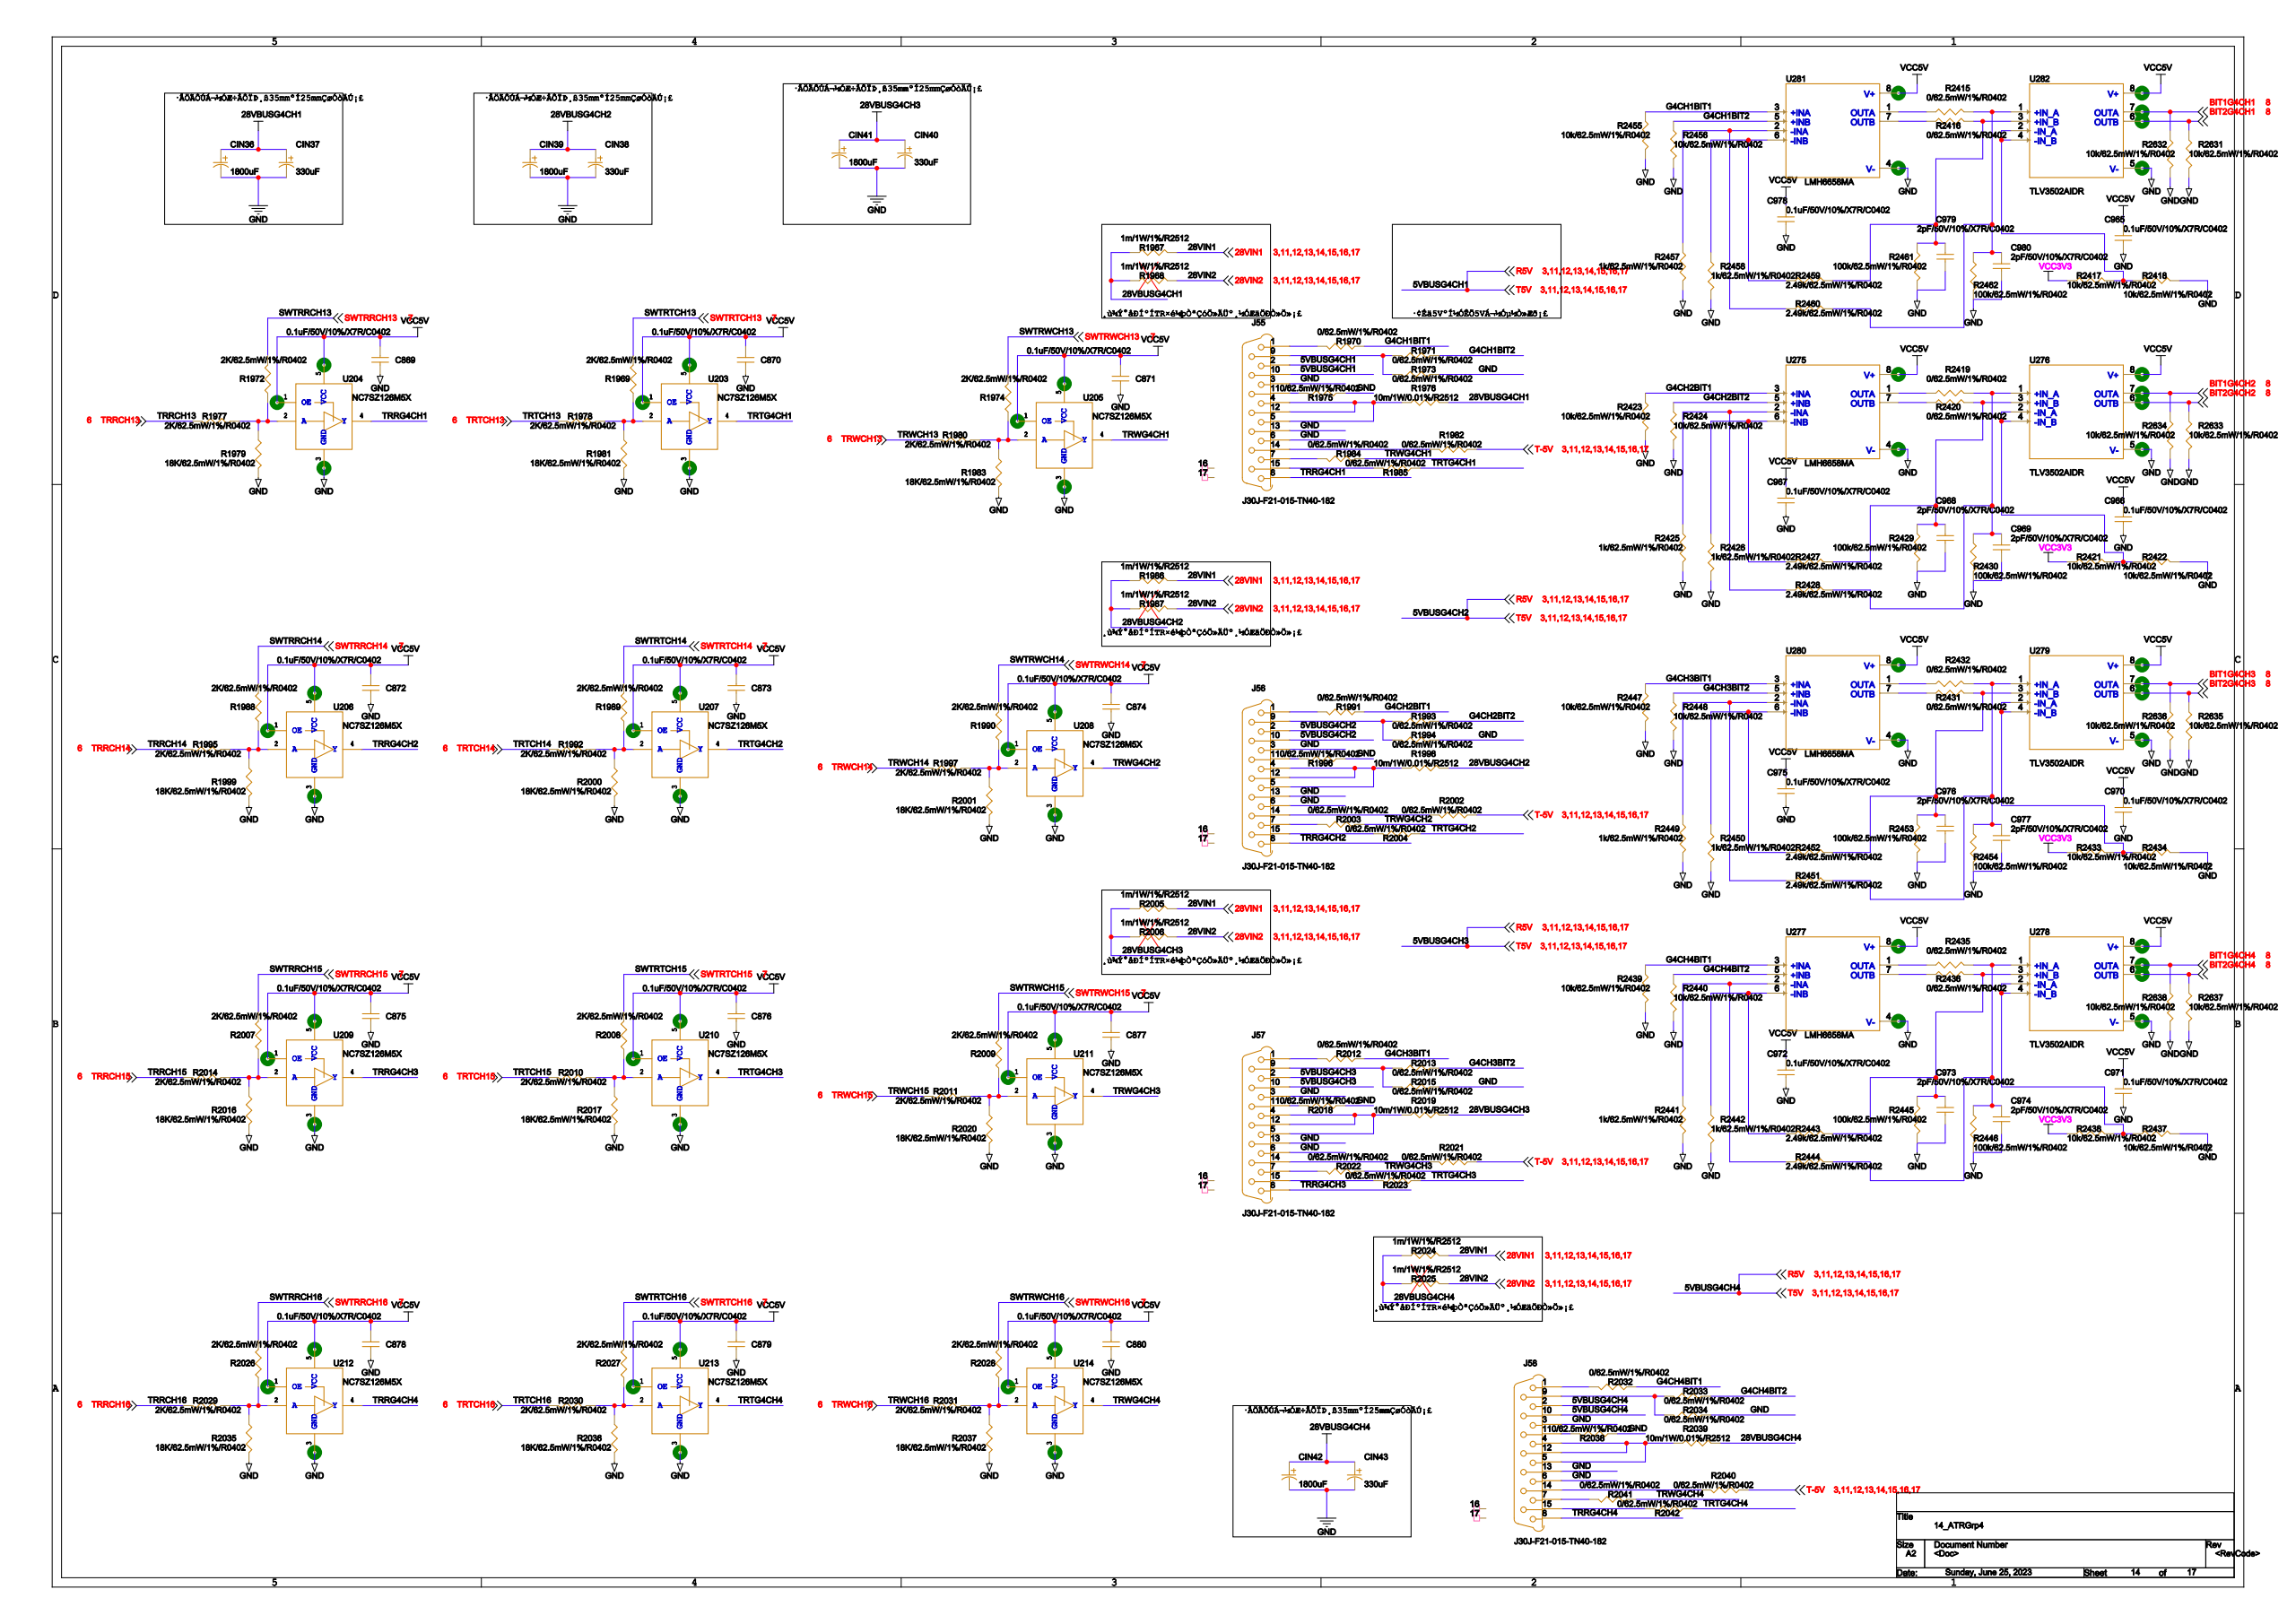Circuit board | Cadence Allegro | 1997 parts | 1536 nets | one sheet of the schematic
Parts on this sheet (reference | value | footprint):
C869 | 0.1uF/50V/10%/X7R/C0402 | 0402
C870 | 0.1uF/50V/10%/X7R/C0402 | 0402
C871 | 0.1uF/50V/10%/X7R/C0402 | 0402
C872 | 0.1uF/50V/10%/X7R/C0402 | 0402
C873 | 0.1uF/50V/10%/X7R/C0402 | 0402
C874 | 0.1uF/50V/10%/X7R/C0402 | 0402
C875 | 0.1uF/50V/10%/X7R/C0402 | 0402
C876 | 0.1uF/50V/10%/X7R/C0402 | 0402
C877 | 0.1uF/50V/10%/X7R/C0402 | 0402
C878 | 0.1uF/50V/10%/X7R/C0402 | 0402
C879 | 0.1uF/50V/10%/X7R/C0402 | 0402
C880 | 0.1uF/50V/10%/X7R/C0402 | 0402
C965 | 0.1uF/50V/10%/X7R/C0402 | 0402
C966 | 0.1uF/50V/10%/X7R/C0402 | 0402
C968 | 2pF/50V/10%/X7R/C0402 | 0402
C969 | 2pF/50V/10%/X7R/C0402 | 0402
C970 | 0.1uF/50V/10%/X7R/C0402 | 0402
C971 | 0.1uF/50V/10%/X7R/C0402 | 0402
C973 | 2pF/50V/10%/X7R/C0402 | 0402
C974 | 2pF/50V/10%/X7R/C0402 | 0402
C976 | 2pF/50V/10%/X7R/C0402 | 0402
C977 | 2pF/50V/10%/X7R/C0402 | 0402
C979 | 2pF/50V/10%/X7R/C0402 | 0402
C980 | 2pF/50V/10%/X7R/C0402 | 0402
CIN36 | ECF1HM182M27OTPO | AP-SMD_BD18-L27-W6_6-LS7_21
CIN37 | ECF1JM331G20OTPO | AP-SMD_BD10-L20-W6_6-LS7_21
CIN38 | ECF1JM331G20OTPO | AP-SMD_BD10-L20-W6_6-LS7_21
CIN39 | ECF1HM182M27OTPO | AP-SMD_BD18-L27-W6_6-LS7_21
CIN40 | ECF1JM331G20OTPO | AP-SMD_BD10-L20-W6_6-LS7_21
CIN41 | ECF1HM182M27OTPO | AP-SMD_BD18-L27-W6_6-LS7_21
CIN42 | ECF1HM182M27OTPO | AP-SMD_BD18-L27-W6_6-LS7_21
CIN43 | ECF1JM331G20OTPO | AP-SMD_BD10-L20-W6_6-LS7_21
J55 | J30J-F21-015-TN40-182 | J30J-F21-015-TN40-182
J56 | J30J-F21-015-TN40-182 | J30J-F21-015-TN40-182
J57 | J30J-F21-015-TN40-182 | J30J-F21-015-TN40-182
J58 | J30J-F21-015-TN40-182 | J30J-F21-015-TN40-182
R1967 | 1m/1W/1%/R2512 | 2512
R1968 | 1m/1W/1%/R2512 | 2512
R1969 | 2K/62.5mW/1%/R0402 | 0402
R1970 | 0/62.5mW/1%/R0402 | 0402
R1971 | 0/62.5mW/1%/R0402 | 0402
R1972 | 2K/62.5mW/1%/R0402 | 0402
R1973 | 0/62.5mW/1%/R0402 | 0402
R1974 | 2K/62.5mW/1%/R0402 | 0402
R1975 | 0/62.5mW/1%/R0402 | 0402
R1976 | 10m/1W/0.01%/R2512 | 2512
R1977 | 2K/62.5mW/1%/R0402 | 0402
R1978 | 2K/62.5mW/1%/R0402 | 0402
R1979 | 18K/62.5mW/1%/R0402 | 0402
R1980 | 2K/62.5mW/1%/R0402 | 0402
R1981 | 18K/62.5mW/1%/R0402 | 0402
R1982 | 0/62.5mW/1%/R0402 | 0402
R1983 | 18K/62.5mW/1%/R0402 | 0402
R1984 | 0/62.5mW/1%/R0402 | 0402
R1985 | 0/62.5mW/1%/R0402 | 0402
R1986 | 1m/1W/1%/R2512 | 2512
R1987 | 1m/1W/1%/R2512 | 2512
R1988 | 2K/62.5mW/1%/R0402 | 0402
R1989 | 2K/62.5mW/1%/R0402 | 0402
R1990 | 2K/62.5mW/1%/R0402 | 0402
R1991 | 0/62.5mW/1%/R0402 | 0402
R1992 | 2K/62.5mW/1%/R0402 | 0402
R1993 | 0/62.5mW/1%/R0402 | 0402
R1994 | 0/62.5mW/1%/R0402 | 0402
R1995 | 2K/62.5mW/1%/R0402 | 0402
R1996 | 0/62.5mW/1%/R0402 | 0402
R1997 | 2K/62.5mW/1%/R0402 | 0402
R1998 | 10m/1W/0.01%/R2512 | 2512
R1999 | 18K/62.5mW/1%/R0402 | 0402
R2000 | 18K/62.5mW/1%/R0402 | 0402
R2001 | 18K/62.5mW/1%/R0402 | 0402
R2002 | 0/62.5mW/1%/R0402 | 0402
R2003 | 0/62.5mW/1%/R0402 | 0402
R2004 | 0/62.5mW/1%/R0402 | 0402
R2005 | 1m/1W/1%/R2512 | 2512
R2006 | 1m/1W/1%/R2512 | 2512
R2007 | 2K/62.5mW/1%/R0402 | 0402
R2008 | 2K/62.5mW/1%/R0402 | 0402
R2009 | 2K/62.5mW/1%/R0402 | 0402
R2010 | 2K/62.5mW/1%/R0402 | 0402
R2011 | 2K/62.5mW/1%/R0402 | 0402
R2012 | 0/62.5mW/1%/R0402 | 0402
R2013 | 0/62.5mW/1%/R0402 | 0402
R2014 | 2K/62.5mW/1%/R0402 | 0402
R2015 | 0/62.5mW/1%/R0402 | 0402
R2016 | 18K/62.5mW/1%/R0402 | 0402
R2017 | 18K/62.5mW/1%/R0402 | 0402
R2018 | 0/62.5mW/1%/R0402 | 0402
R2019 | 10m/1W/0.01%/R2512 | 2512
R2020 | 18K/62.5mW/1%/R0402 | 0402
R2021 | 0/62.5mW/1%/R0402 | 0402
R2022 | 0/62.5mW/1%/R0402 | 0402
R2023 | 0/62.5mW/1%/R0402 | 0402
R2024 | 1m/1W/1%/R2512 | 2512
R2025 | 1m/1W/1%/R2512 | 2512
R2026 | 2K/62.5mW/1%/R0402 | 0402
R2027 | 2K/62.5mW/1%/R0402 | 0402
R2028 | 2K/62.5mW/1%/R0402 | 0402
R2029 | 2K/62.5mW/1%/R0402 | 0402
R2030 | 2K/62.5mW/1%/R0402 | 0402
R2031 | 2K/62.5mW/1%/R0402 | 0402
R2032 | 0/62.5mW/1%/R0402 | 0402
R2033 | 0/62.5mW/1%/R0402 | 0402
R2034 | 0/62.5mW/1%/R0402 | 0402
R2035 | 18K/62.5mW/1%/R0402 | 0402
R2036 | 18K/62.5mW/1%/R0402 | 0402
R2037 | 18K/62.5mW/1%/R0402 | 0402
R2038 | 0/62.5mW/1%/R0402 | 0402
R2039 | 10m/1W/0.01%/R2512 | 2512
R2040 | 0/62.5mW/1%/R0402 | 0402
R2041 | 0/62.5mW/1%/R0402 | 0402
R2042 | 0/62.5mW/1%/R0402 | 0402
R2415 | 0/62.5mW/1%/R0402 | 0402
R2416 | 0/62.5mW/1%/R0402 | 0402
R2417 | 10k/62.5mW/1%/R0402 | 0402
R2418 | 10k/62.5mW/1%/R0402 | 0402
R2419 | 0/62.5mW/1%/R0402 | 0402
R2420 | 0/62.5mW/1%/R0402 | 0402
R2421 | 10k/62.5mW/1%/R0402 | 0402
R2422 | 10k/62.5mW/1%/R0402 | 0402
R2423 | 10k/62.5mW/1%/R0402 | 0402
R2424 | 10k/62.5mW/1%/R0402 | 0402
R2425 | 1K/62.5mW/1%/R0402 | 0402
R2426 | 1K/62.5mW/1%/R0402 | 0402
R2428 | 2.49k/62.5mW/1%/R0402 | 0402
R2429 | 100k/62.5mW/1%/R0402 | 0402
R2430 | 100k/62.5mW/1%/R0402 | 0402
R2431 | 0/62.5mW/1%/R0402 | 0402
R2432 | 0/62.5mW/1%/R0402 | 0402
R2433 | 10k/62.5mW/1%/R0402 | 0402
R2434 | 10k/62.5mW/1%/R0402 | 0402
R2435 | 0/62.5mW/1%/R0402 | 0402
R2436 | 0/62.5mW/1%/R0402 | 0402
R2437 | 10k/62.5mW/1%/R0402 | 0402
R2438 | 10k/62.5mW/1%/R0402 | 0402
R2439 | 10k/62.5mW/1%/R0402 | 0402
R2440 | 10k/62.5mW/1%/R0402 | 0402
R2441 | 1K/62.5mW/1%/R0402 | 0402
R2442 | 1K/62.5mW/1%/R0402 | 0402
R2444 | 2.49k/62.5mW/1%/R0402 | 0402
R2445 | 100k/62.5mW/1%/R0402 | 0402
R2446 | 100k/62.5mW/1%/R0402 | 0402
R2447 | 10k/62.5mW/1%/R0402 | 0402
R2448 | 10k/62.5mW/1%/R0402 | 0402
R2449 | 1K/62.5mW/1%/R0402 | 0402
R2450 | 1K/62.5mW/1%/R0402 | 0402
R2451 | 2.49k/62.5mW/1%/R0402 | 0402
R2452 | 2.49k/62.5mW/1%/R0402 | 0402
R2453 | 100k/62.5mW/1%/R0402 | 0402
R2454 | 100k/62.5mW/1%/R0402 | 0402
R2455 | 10k/62.5mW/1%/R0402 | 0402
R2456 | 10k/62.5mW/1%/R0402 | 0402
R2457 | 1K/62.5mW/1%/R0402 | 0402
R2458 | 1K/62.5mW/1%/R0402 | 0402
R2460 | 2.49k/62.5mW/1%/R0402 | 0402
R2461 | 100k/62.5mW/1%/R0402 | 0402
R2462 | 100k/62.5mW/1%/R0402 | 0402
R2631 | 10k/62.5mW/1%/R0402 | 0402
R2632 | 10k/62.5mW/1%/R0402 | 0402
R2633 | 10k/62.5mW/1%/R0402 | 0402
R2634 | 10k/62.5mW/1%/R0402 | 0402
R2635 | 10k/62.5mW/1%/R0402 | 0402
R2636 | 10k/62.5mW/1%/R0402 | 0402
R2637 | 10k/62.5mW/1%/R0402 | 0402
R2638 | 10k/62.5mW/1%/R0402 | 0402
U203 | NC7SZ126M5X | SOT-23-5
U204 | NC7SZ126M5X | SOT-23-5
U205 | NC7SZ126M5X | SOT-23-5
U206 | NC7SZ126M5X | SOT-23-5
U207 | NC7SZ126M5X | SOT-23-5
U208 | NC7SZ126M5X | SOT-23-5
U209 | NC7SZ126M5X | SOT-23-5
U210 | NC7SZ126M5X | SOT-23-5
U211 | NC7SZ126M5X | SOT-23-5
U212 | NC7SZ126M5X | SOT-23-5
U213 | NC7SZ126M5X | SOT-23-5
U214 | NC7SZ126M5X | SOT-23-5
U275 | LMH6658MA | SOIC127P599X175-8N
U277 | LMH6658MA | SOIC127P599X175-8N
U279 | TLV3502AIDR | SOIC127P599X175-8N
U281 | LMH6658MA | SOIC127P599X175-8N
Nets of these parts (net: part-pin ...):
3.3V: R2417-1 R2421-1 R2433-1 R2438-1
AGND: C869-2 C870-2 C871-2 C872-2 C873-2 C874-2 C875-2 C876-2 C877-2 C878-2 C879-2 C880-2 C965-2 C966-2 C968-2 C969-2 C970-2 C971-2 C973-2 C974-2 C976-2 C977-2 C979-2 C980-2 CIN36-2 CIN37-2 CIN38-2 CIN39-2 CIN40-2 CIN41-2 CIN42-2 CIN43-2 J55-3 J55-6 J55-13 J56-3 J56-6 J56-13 J57-3 J57-6 J57-13 J58-3 J58-6 J58-13 R1973-1 R1975-1 R1979-1 R1981-1 R1983-1 R1994-1 R1996-1 R1999-1 R2000-1 R2001-1 R2015-1 R2016-1 R2017-1 R2018-1 R2020-1 R2034-1 R2035-1 R2036-1 R2037-1 R2038-1 R2418-2 R2422-2 R2423-2 R2424-2 R2425-2 R2426-2 R2429-2 R2430-2 R2434-2 R2437-2 R2439-2 R2440-2 R2441-2 R2442-2 R2445-2 R2446-2 R2447-2 R2448-2 R2449-2 R2450-2 R2453-2 R2454-2 R2455-2 R2456-2 R2457-2 R2458-2 R2461-2 R2462-2 R2631-2 R2632-2 R2633-2 R2634-2 R2635-2 R2636-2 R2637-2 R2638-2 U203-3 U204-3 U205-3 U206-3 U207-3 U208-3 U209-3 U210-3 U211-3 U212-3 U213-3 U214-3 U275-4 U277-4 U279-5 U281-4
VCC5V: C869-1 C870-1 C871-1 C872-1 C873-1 C874-1 C875-1 C876-1 C877-1 C878-1 C879-1 C880-1 C965-1 C966-1 C970-1 C971-1 U203-1 U203-5 U204-1 U204-5 U205-1 U205-5 U206-1 U206-5 U207-1 U207-5 U208-1 U208-5 U209-1 U209-5 U210-1 U210-5 U211-1 U211-5 U212-1 U212-5 U213-1 U213-5 U214-1 U214-5 U275-8 U277-8 U279-8 U281-8
N24402779: R2426-1 U275-6
N24402789: C968-1 R2420-2 R2429-1
N24402767: R2425-1 R2428-1 U275-2
N24402787: C969-1 R2419-2 R2428-2 R2430-1
N24403333: R2442-1 U277-6
N24403343: C973-1 R2436-2 R2445-1
N24403321: R2441-1 R2444-1 U277-2
N24403341: C974-1 R2435-2 R2444-2 R2446-1
N24403145: R2449-1 R2451-1
N24403161: C977-1 R2432-2 R2451-2 R2454-1 U279-1
N24403149: R2450-1 R2452-1
N24403163: C976-1 R2431-2 R2452-2 R2453-1 U279-3
N24402599: R2458-1 U281-6
N24402609: C979-1 R2416-2 R2461-1
N24402595: R2457-1 R2460-1 U281-2
N24402607: C980-1 R2415-2 R2460-2 R2462-1
G4CH2BIT1: R1991-1 R2423-1 U275-3
G4CH2BIT2: R1993-1 R2424-1 U275-5
N24402783: R2419-1 U275-1
N24402785: R2420-1 U275-7
G4CH4BIT1: R2032-1 R2439-1 U277-3
G4CH4BIT2: R2033-1 R2440-1 U277-5
N24403337: R2435-1 U277-1
N24403339: R2436-1 U277-7
G4CH3BIT1: R2012-1 R2447-1
G4CH3BIT2: R2013-1 R2448-1
N24403157: R2432-1
N24403159: R2431-1
G4CH1BIT1: R1970-1 R2455-1 U281-3
G4CH1BIT2: R1971-1 R2456-1 U281-5
N24402603: R2415-1 U281-1
N24402605: R2416-1 U281-7
N24402841: R2421-2 R2422-1
BIT1G4CH2: R2634-1
BIT2G4CH2: R2633-1
N24403395: R2437-1 R2438-2
BIT1G4CH4: R2638-1
BIT2G4CH4: R2637-1
N24403215: R2433-2 R2434-1 U279-2 U279-4
BIT1G4CH3: R2636-1 U279-7
BIT2G4CH3: R2635-1 U279-6
N24402661: R2417-2 R2418-1
BIT1G4CH1: R2632-1
BIT2G4CH1: R2631-1
R5V: J55-2 J55-10 J56-2 J56-10 J57-2 J57-10 J58-2 J58-10
N23728226: J55-1 R1970-2
N23728239: J55-11 R1975-2
N23728241: J55-4 J55-5 J55-12 R1976-1
N23728253: J55-14 R1982-2
N23728257: J55-15 R1985-2
N23728255: J55-7 R1984-2
TRRG4CH1: J55-8 U204-4
N23728228: J55-9 R1971-2 R1973-2
N23728785: J56-1 R1991-2
N23728798: J56-11 R1996-2
N23728800: J56-4 J56-5 J56-12 R1998-1
N23728812: J56-14 R2002-2
N23728816: J56-15 R2004-2
N23728814: J56-7 R2003-2
TRRG4CH2: J56-8 U206-4
N23728787: J56-9 R1993-2 R1994-2
N23729412: J57-1 R2012-2
N23729425: J57-11 R2018-2
N23729427: J57-4 J57-5 J57-12 R2019-1
N23729439: J57-14 R2021-2
N23729443: J57-15 R2023-2
N23729441: J57-7 R2022-2
TRRG4CH3: J57-8 U209-4
N23729414: J57-9 R2013-2 R2015-2
N23730216: J58-1 R2032-2
N23730229: J58-11 R2038-2
N23730231: J58-4 J58-5 J58-12 R2039-1
N23730243: J58-14 R2040-2
N23730247: J58-15 R2042-2
N23730245: J58-7 R2041-2
TRRG4CH4: J58-8 U212-4
N23730218: J58-9 R2033-2 R2034-2
28VIN1: R1967-2 R1986-2 R2005-2 R2024-2
T-5V: R1982-1 R2002-1 R2021-1 R2040-1
28VIN2: R1968-2 R1987-2 R2006-2 R2025-2
28VBUSG4CH1: CIN36-1 CIN37-1 R1967-1 R1968-1 R1976-2
28VBUSG4CH2: CIN38-1 CIN39-1 R1986-1 R1987-1 R1998-2
28VBUSG4CH3: CIN40-1 CIN41-1 R2005-1 R2006-1 R2019-2
28VBUSG4CH4: CIN42-1 CIN43-1 R2024-1 R2025-1 R2039-2
SWTRTCH13: R1969-1
N24010050: R1969-2 R1978-2 R1981-2 U203-2
SWTRRCH13: R1972-1
N24011030: R1972-2 R1977-2 R1979-2 U204-2
SWTRWCH13: R1974-1
N24010538: R1974-2 R1980-2 R1983-2 U205-2
TRRCH13: R1977-1
TRTCH13: R1978-1
TRWCH13: R1980-1
SWTRRCH14: R1988-1
N24011148: R1988-2 R1995-2 R1999-2 U206-2
SWTRTCH14: R1989-1
N24010168: R1989-2 R1992-2 R2000-2 U207-2
SWTRWCH14: R1990-1
N24010660: R1990-2 R1997-2 R2001-2 U208-2
TRTCH14: R1992-1
TRRCH14: R1995-1
TRWCH14: R1997-1
SWTRRCH15: R2007-1
N24011274: R2007-2 R2014-2 R2016-2 U209-2
SWTRTCH15: R2008-1
N24010294: R2008-2 R2010-2 R2017-2 U210-2
SWTRWCH15: R2009-1
N24010782: R2009-2 R2011-2 R2020-2 U211-2
TRTCH15: R2010-1
TRWCH15: R2011-1
TRRCH15: R2014-1
SWTRRCH16: R2026-1
N24011392: R2026-2 R2029-2 R2035-2 U212-2
SWTRTCH16: R2027-1
N24010416: R2027-2 R2030-2 R2036-2 U213-2
SWTRWCH16: R2028-1
N24010904: R2028-2 R2031-2 R2037-2 U214-2
TRRCH16: R2029-1
TRTCH16: R2030-1
TRWCH16: R2031-1
TRTG4CH1: R1985-1 U203-4
TRWG4CH1: R1984-1 U205-4
TRTG4CH2: R2004-1 U207-4
TRWG4CH2: R2003-1 U208-4
TRTG4CH3: R2023-1 U210-4
TRWG4CH3: R2022-1 U211-4
TRTG4CH4: R2042-1 U213-4
TRWG4CH4: R2041-1 U214-4